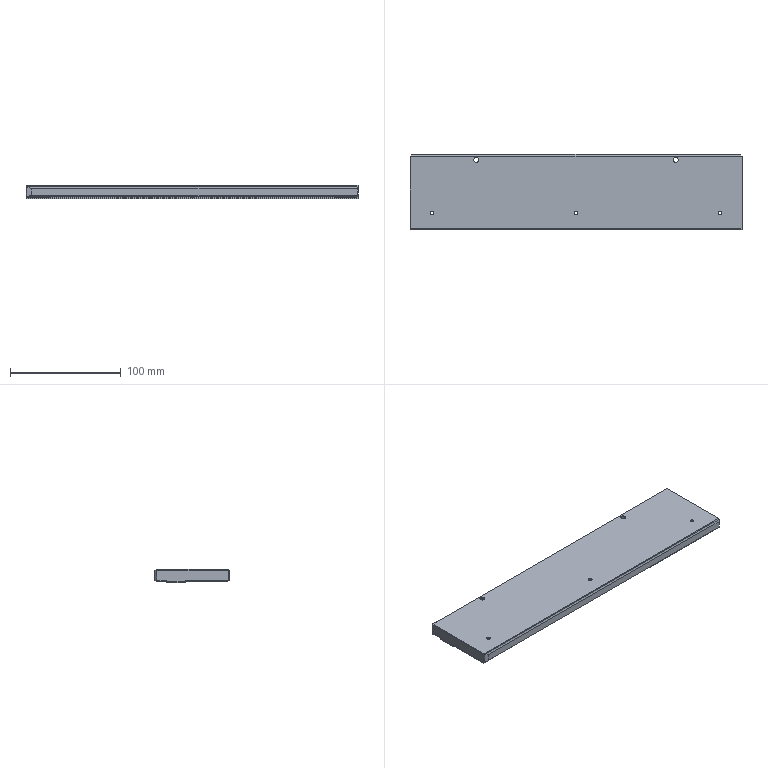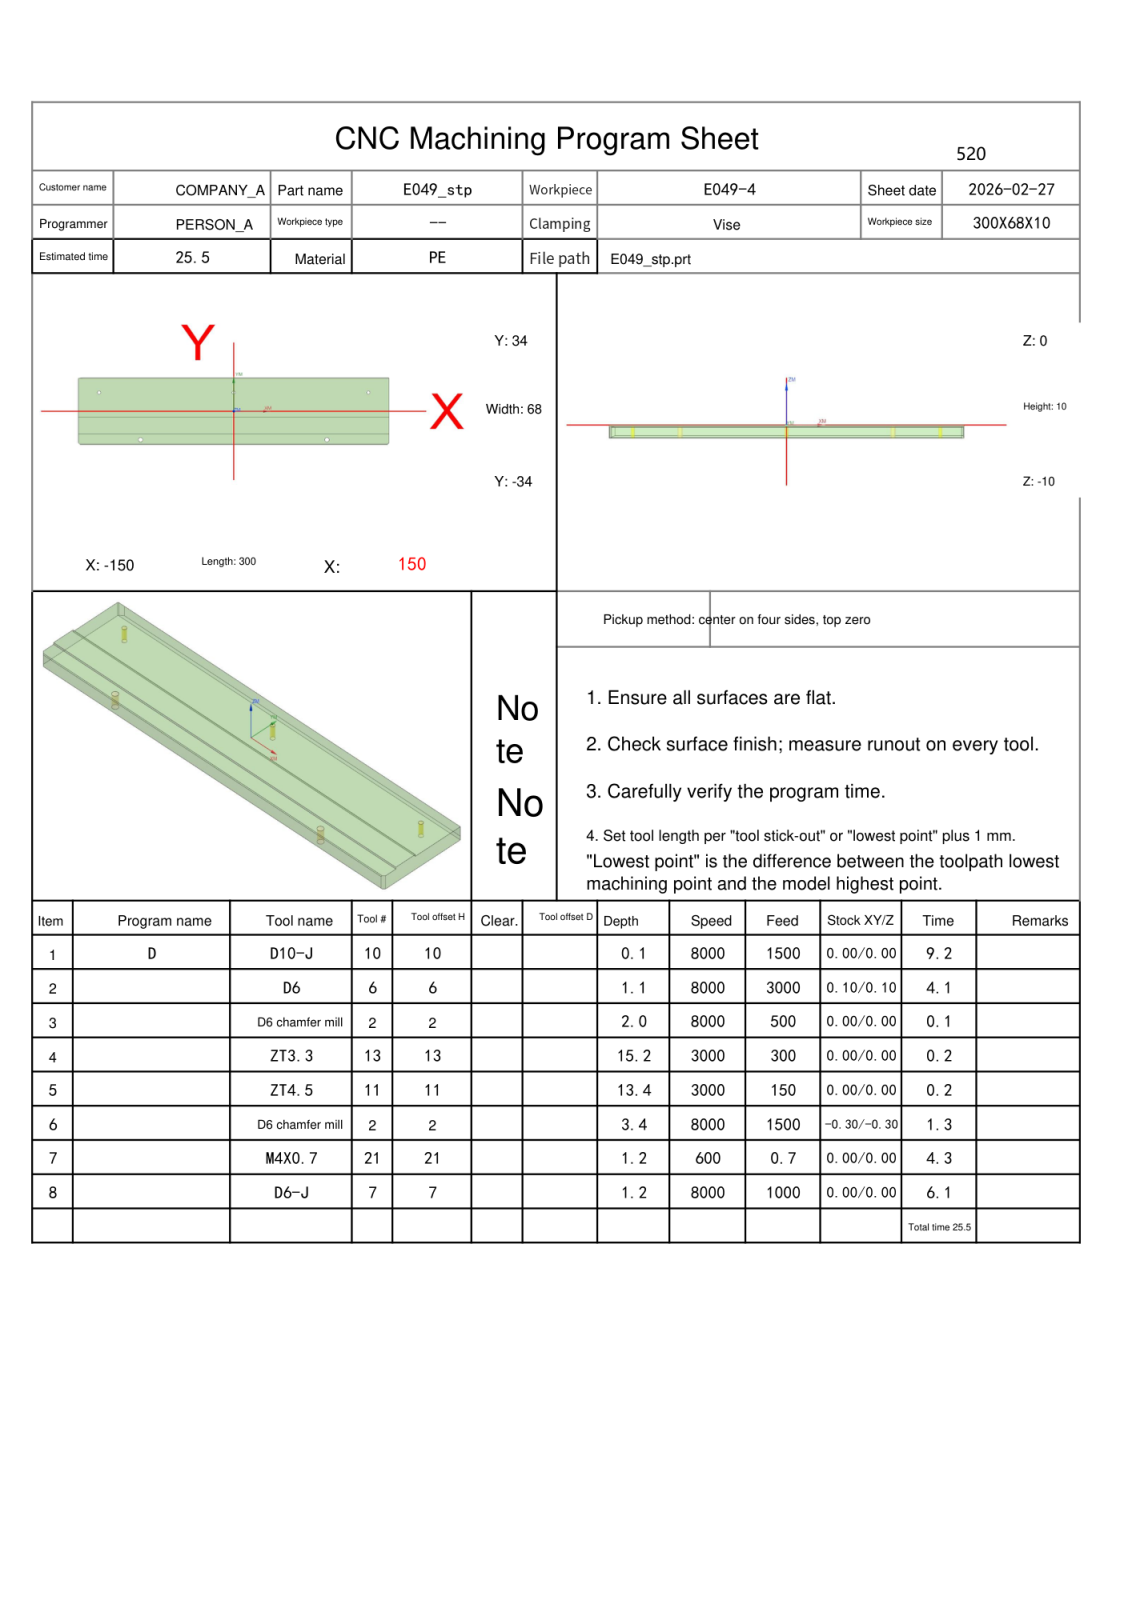NC program | NX | posted by the shop | part box 300 x 68 x 12 mm
Whole program:
%
O0001
(Machine time: 27.03 MIN)
(===Total Tool:7===)
(T10=D10-J  D=10.  R=0.   D-  H10 Z=0.    )
(T6=D6      D=6.   R=0.   D-  H06 Z=-1.1  )
(T2=D6 chamfer mill   D=6.   R=0.   D-  H02 Z=-3.37 )
(T13=ZT3.3  D=3.3  DR_a=118 D-  H13 Z=-15.2 )
(T11=ZT4.5  D=4.5  DR_a=118 D-  H11 Z=-13.35)
(T21=M4X0.7 D=3.3  DR_a=180 D-  H21 Z=-1.2  )
(T7=D6-J    D=6.   R=0.   D7  H07 Z=-1.2  )
G80 G90 G17 G49 G40
G91 G28 Z0
M01
N1 T10 M06
(D10-J  D=10. R=0. H=10 ce=0.00 di=0.10)
G00 G90 G54 X140.3 Y44. M03 S4500
G43 H10 Z30.
M08
Z2.55
G01 Z.55 F1500.
X145.3 Y39.
X155. Y29.3
Y19.6
X135.6 Y39.
X125.9
X155. Y9.9
Y.2
X116.2 Y39.
X106.5
X155. Y-9.5
Y-19.2
X96.8 Y39.
X87.1
X155. Y-28.9
Y-38.6
X77.4 Y39.
X67.7
X145.7 Y-39.
X136.
X58. Y39.
X48.3
X126.3 Y-39.
X116.6
X38.6 Y39.
X28.9
X106.9 Y-39.
X97.2
X19.2 Y39.
X9.5
X87.5 Y-39.
X77.8
X-.2 Y39.
X-9.9
X68.1 Y-39.
X58.4
X-19.6 Y39.
X-29.3
X48.7 Y-39.
X39.
X-39. Y39.
X-48.7
X29.3 Y-39.
X19.6
X-58.4 Y39.
X-68.1
X9.9 Y-39.
X.2
X-77.8 Y39.
X-87.5
X-9.5 Y-39.
X-19.2
X-97.2 Y39.
X-106.9
X-28.9 Y-39.
X-38.6
X-116.6 Y39.
X-126.3
X-48.3 Y-39.
X-58.
X-136. Y39.
X-145.7
X-67.7 Y-39.
X-77.4
X-155. Y38.6
Y28.9
X-87.1 Y-39.
X-96.8
X-155. Y19.2
Y9.5
X-106.5 Y-39.
X-116.2
X-155. Y-.2
Y-9.9
X-125.9 Y-39.
X-135.6
X-155. Y-19.6
Y-29.3
X-145.3 Y-39.
X-140.3 Y-44.
Z2.55
G00 Z4.
X160. Y24.3
Z2.1
G01 Z.1
X155. Y29.3
X145.3 Y39.
X135.6
X155. Y19.6
Y9.9
X125.9 Y39.
X116.2
X155. Y.2
Y-9.5
X106.5 Y39.
X96.8
X155. Y-19.2
Y-28.9
X87.1 Y39.
X77.4
X155. Y-38.6
Y-39.
X145.7
X67.7 Y39.
X58.
X136. Y-39.
X126.3
X48.3 Y39.
X38.6
X116.6 Y-39.
X106.9
X28.9 Y39.
X19.2
X97.2 Y-39.
X87.5
X9.5 Y39.
X-.2
X77.8 Y-39.
X68.1
X-9.9 Y39.
X-19.6
X58.4 Y-39.
X48.7
X-29.3 Y39.
X-39.
X39. Y-39.
X29.3
X-48.7 Y39.
X-58.4
X19.6 Y-39.
X9.9
X-68.1 Y39.
X-77.8
X.2 Y-39.
X-9.5
X-87.5 Y39.
X-97.2
X-19.2 Y-39.
X-28.9
X-106.9 Y39.
X-116.6
X-38.6 Y-39.
X-48.3
X-126.3 Y39.
X-136.
X-58. Y-39.
X-67.7
X-145.7 Y39.
X-155.
Y38.6
X-77.4 Y-39.
X-87.1
X-155. Y28.9
Y19.2
X-96.8 Y-39.
X-106.5
X-155. Y9.5
Y-.2
X-116.2 Y-39.
X-125.9
X-155. Y-9.9
Y-19.6
X-135.6 Y-39.
X-145.3
X-155. Y-29.3
X-160. Y-24.3
Z2.1
G00 Z30.
G00 G90 X-167. Y17.3 M03 S8000
Z30.
Z2.
G01 Z0.0 F1000.
X-155. Y29.3
X-145.3 Y39.
X-135.6
X-155. Y19.6
Y9.9
X-125.9 Y39.
X-116.2
X-155. Y.2
Y-9.5
X-106.5 Y39.
X-96.8
X-155. Y-19.2
Y-28.9
X-87.1 Y39.
X-77.4
X-155. Y-38.6
Y-39.
X-145.7
X-67.7 Y39.
X-58.
X-136. Y-39.
X-126.3
X-48.3 Y39.
X-38.6
X-116.6 Y-39.
X-106.9
X-28.9 Y39.
X-19.2
X-97.2 Y-39.
X-87.5
X-9.5 Y39.
X.2
X-77.8 Y-39.
X-68.1
X9.9 Y39.
X19.6
X-58.4 Y-39.
X-48.7
X29.3 Y39.
X39.
X-39. Y-39.
X-29.3
X48.7 Y39.
X58.4
X-19.6 Y-39.
X-9.9
X68.1 Y39.
X77.8
X-.2 Y-39.
X9.5
X87.5 Y39.
X97.2
X19.2 Y-39.
X28.9
X106.9 Y39.
X116.6
X38.6 Y-39.
X48.3
X126.3 Y39.
X136.
X58. Y-39.
X67.7
X145.7 Y39.
X155.
Y38.6
X77.4 Y-39.
X87.1
X155. Y28.9
Y19.2
X96.8 Y-39.
X106.5
X155. Y9.5
Y-.2
X116.2 Y-39.
X125.9
X155. Y-9.9
Y-19.6
X135.6 Y-39.
X145.3
X155. Y-29.3
X167. Y-17.3
Z2.
G00 Z30.
G91 G28 Z0.0
M05
M09
G91 G28 Z0.0
M01
N2 T06 M06
(D6  D=6. R=0. H=06 ce=0.10 di=0.10)
G00 G90 G54 X156. Y36.1 M03 S8000
G43 H06 Z11.
M08
Z1.133
G01 Z-.367 F3000.
X152.94
X-150.894
G03 X-151.338 Y35.903 I.001 J-.6
G01 X-152.785 Y34.304
G03 X-152.94 Y33.902 I.445 J-.402
G01 Y33.699
G03 X-152.341 Y33.1 I.6 J.001
G01 X152.341
G02 X152.94 Y32.501 I-.001 J-.6
G01 Y29.199
G02 X152.341 Y28.6 I-.6 J.001
G01 X-152.341
G03 X-152.94 Y28.001 I.001 J-.6
G01 Y24.699
G03 X-152.341 Y24.1 I.6 J.001
G01 X152.341
G02 X152.94 Y23.501 I-.001 J-.6
G01 Y20.199
G02 X152.341 Y19.6 I-.6 J.001
G01 X-152.341
G03 X-152.94 Y19.001 I.001 J-.6
G01 Y15.699
G03 X-152.341 Y15.1 I.6 J.001
G01 X152.341
G02 X152.94 Y14.501 I-.001 J-.6
G01 Y11.199
G02 X152.341 Y10.6 I-.6 J.001
G01 X-152.341
G03 X-152.94 Y10.001 I.001 J-.6
G01 Y6.699
G03 X-152.341 Y6.1 I.6 J.001
G01 X152.341
G02 X152.94 Y5.501 I-.001 J-.6
G01 Y2.199
G02 X152.341 Y1.6 I-.6 J.001
G01 X-152.427
G03 X-153.019 Y1.093 I.001 J-.6
G01 X-153.533 Y-2.208
X-153.54 Y-2.3
G03 X-152.94 Y-2.9 I.6 J0.0
G01 X152.94
X156.1
Z1.133
G00 X156. Y36.1
Z.767
G01 Z-.733
X152.94
X-150.894
G03 X-151.338 Y35.903 I.001 J-.6
G01 X-152.785 Y34.304
G03 X-152.94 Y33.902 I.445 J-.402
G01 Y33.699
G03 X-152.341 Y33.1 I.6 J.001
G01 X152.341
G02 X152.94 Y32.501 I-.001 J-.6
G01 Y29.199
G02 X152.341 Y28.6 I-.6 J.001
G01 X-152.341
G03 X-152.94 Y28.001 I.001 J-.6
G01 Y24.699
G03 X-152.341 Y24.1 I.6 J.001
G01 X152.341
G02 X152.94 Y23.501 I-.001 J-.6
G01 Y20.199
G02 X152.341 Y19.6 I-.6 J.001
G01 X-152.341
G03 X-152.94 Y19.001 I.001 J-.6
G01 Y15.699
G03 X-152.341 Y15.1 I.6 J.001
G01 X152.341
G02 X152.94 Y14.501 I-.001 J-.6
G01 Y11.199
G02 X152.341 Y10.6 I-.6 J.001
G01 X-152.341
G03 X-152.94 Y10.001 I.001 J-.6
G01 Y6.699
G03 X-152.341 Y6.1 I.6 J.001
G01 X152.341
G02 X152.94 Y5.501 I-.001 J-.6
G01 Y2.199
G02 X152.341 Y1.6 I-.6 J.001
G01 X-152.427
G03 X-153.019 Y1.093 I.001 J-.6
G01 X-153.533 Y-2.208
X-153.54 Y-2.3
G03 X-152.94 Y-2.9 I.6 J0.0
G01 X152.94
X156.1
Z.767
G00 X156. Y36.1
Z.4
G01 Z-1.1
X152.94
X-150.894
G03 X-151.338 Y35.903 I.001 J-.6
G01 X-152.785 Y34.304
G03 X-152.94 Y33.902 I.445 J-.402
G01 Y33.699
G03 X-152.341 Y33.1 I.6 J.001
G01 X152.341
G02 X152.94 Y32.501 I-.001 J-.6
G01 Y29.199
G02 X152.341 Y28.6 I-.6 J.001
G01 X-152.341
G03 X-152.94 Y28.001 I.001 J-.6
G01 Y24.699
G03 X-152.341 Y24.1 I.6 J.001
G01 X152.341
G02 X152.94 Y23.501 I-.001 J-.6
G01 Y20.199
G02 X152.341 Y19.6 I-.6 J.001
G01 X-152.341
G03 X-152.94 Y19.001 I.001 J-.6
G01 Y15.699
G03 X-152.341 Y15.1 I.6 J.001
G01 X152.341
G02 X152.94 Y14.501 I-.001 J-.6
G01 Y11.199
G02 X152.341 Y10.6 I-.6 J.001
G01 X-152.341
G03 X-152.94 Y10.001 I.001 J-.6
G01 Y6.699
G03 X-152.341 Y6.1 I.6 J.001
G01 X152.341
G02 X152.94 Y5.501 I-.001 J-.6
G01 Y2.199
G02 X152.341 Y1.6 I-.6 J.001
G01 X-152.427
G03 X-153.019 Y1.093 I.001 J-.6
G01 X-153.533 Y-2.208
X-153.54 Y-2.3
G03 X-152.94 Y-2.9 I.6 J0.0
G01 X152.94
X156.1
Z.4
G00 Z3.
X155.353 Y-35.1
Z1.133
G01 Z-.367
X151.058
X-150.81
G02 X-151.233 Y-34.925 I.001 J.6
G01 X-152.764 Y-33.393
G02 X-152.94 Y-32.969 I.424 J.424
G01 Y-31.199
G02 X-152.341 Y-30.6 I.6 J-.001
G01 X152.427
G03 X153.019 Y-30.093 I-.001 J.6
G01 X153.533 Y-26.792
X153.54 Y-26.7
G03 X152.94 Y-26.1 I-.6 J0.0
G01 X-152.94
X-156.1
Z1.133
G00 X155.353 Y-35.1
Z.767
G01 Z-.733
X151.058
X-150.81
G02 X-151.233 Y-34.925 I.001 J.6
G01 X-152.764 Y-33.393
G02 X-152.94 Y-32.969 I.424 J.424
G01 Y-31.199
G02 X-152.341 Y-30.6 I.6 J-.001
G01 X152.427
G03 X153.019 Y-30.093 I-.001 J.6
G01 X153.533 Y-26.792
X153.54 Y-26.7
G03 X152.94 Y-26.1 I-.6 J0.0
G01 X-152.94
X-156.1
Z.767
G00 X155.353 Y-35.1
Z.4
G01 Z-1.1
X151.058
X-150.81
G02 X-151.233 Y-34.925 I.001 J.6
G01 X-152.764 Y-33.393
G02 X-152.94 Y-32.969 I.424 J.424
G01 Y-31.199
G02 X-152.341 Y-30.6 I.6 J-.001
G01 X152.427
G03 X153.019 Y-30.093 I-.001 J.6
G01 X153.533 Y-26.792
X153.54 Y-26.7
G03 X152.94 Y-26.1 I-.6 J0.0
G01 X-152.94
X-156.1
Z.4
G00 Z11.
G91 G28 Z0.0
M05
M09
G91 G28 Z0.0
M01
N3 T02 M06
(D6 chamfer mill  D=6. R=0. H=02 ce=0.00 di=0.10)
G00 G90 G54 X130. Y19. M03 S8000
G43 H02 Z30.
M08
G98 G81 X130. Y19. Z-2. R-.2 F500.
X90. Y-29.
X0.0 Y19.
X-90. Y-29.
X-130. Y19.
G80
G00 Z30.
G91 G28 Z0.0
M05
M09
G91 G28 Z0.0
M01
N4 T13 M06
(ZT3.3 D=3.3 DR_a=118 H=13)
G00 G90 G54 X130. Y19. M03 S3000
G43 H13 Z30.
M08
G98 G83 X130. Y19. Z-15.2 R-.2 F300. Q2.
X0.0
X-130.
G80
G00 Z30.
G91 G28 Z0.0
M05
M09
G91 G28 Z0.0
M01
N5 T11 M06
(ZT4.5 D=4.5 DR_a=118 H=11)
G00 G90 G54 X-90. Y-29. M03 S3000
G43 H11 Z30.
M08
G98 G83 X-90. Y-29. Z-13.352 R-.2 F150. Q3.
X90.
G80
G00 Z30.
G91 G28 Z0.0
M05
M09
G91 G28 Z0.0
M01
N6 T02 M06
(D6 chamfer mill  D=6. R=0. H=02 ce=0.00 di=0.10)
G00 G90 G54 X130. Y19. M03 S8000
G43 H02 Z30.
M08
G98 G81 X130. Y19. Z-3.371 R1.8 F500.
X0.0
X-130.
G80
G00 Z30.
G00 G90 X-89.982 Y-29.55 M03 S8000
Z30.
Z-1.7
G01 Z-2.2 F500.
X-89.95 Y-30.5
G03 X-88.45 Y-29. I0.0 J1.5
X-90. Y-27.45 I-1.55 J0.0
X-91.55 Y-29. I0.0 J-1.55
X-90. Y-30.55 I1.55 J0.0
X-88.45 Y-29. I0.0 J1.55
X-89.95 Y-27.5 I-1.5 J0.0
G01 X-89.982 Y-28.45
Z-1.7
G00 Z30.
X90.018 Y-29.55
Z-1.7
G01 Z-2.2
X90.05 Y-30.5
G03 X91.55 Y-29. I0.0 J1.5
X90. Y-27.45 I-1.55 J0.0
X88.45 Y-29. I0.0 J-1.55
X90. Y-30.55 I1.55 J0.0
X91.55 Y-29. I0.0 J1.55
X90.05 Y-27.5 I-1.5 J0.0
G01 X90.018 Y-28.45
Z-1.7
G00 Z30.
G00 G90 X.386 Y-23.827 M03 S6500
Z30.
Z.572
G01 Z-.8 F1500.
G03 X.1 Y-23.627 I-1.286 J-1.532
G01 X.054 Y-23.597
X0.0 Y-23.6
X-150.
G02 X-150.6 Y-23. I0.0 J.6
G01 Y-6.
G02 X-150. Y-5.4 I.6 J0.0
G01 X150.
G02 X150.6 Y-6. I0.0 J-.6
G01 Y-23.
G02 X150. Y-23.6 I-.6 J0.0
G01 X0.0
X-.054 Y-23.597
X-.1 Y-23.627
G03 X-.386 Y-23.827 I1. J-1.732
G01 Z.572
G00 Z10.
X150.6 Y-24.898
Z2.
G01 Z-2.
Y-32.
X150.58 Y-32.155
X150.52 Y-32.3
X150.424 Y-32.424
X148.924 Y-33.924
X148.8 Y-34.02
X148.691 Y-34.065
X148.667 Y-34.083
X148.611 Y-34.172
Z-.482
G00 Z10.
X-148.611
Z-.482
G01 Z-2.
X-148.667 Y-34.083
X-148.691 Y-34.065
X-148.8 Y-34.02
X-148.924 Y-33.924
X-150.424 Y-32.424
X-150.52 Y-32.3
X-150.58 Y-32.155
X-150.6 Y-32.
Y-24.898
Z2.
G00 Z10.
X-88.535 Y-29.407
Z-.521
G01 Z-2.
G03 X-88.366 Y-29.102 I-1.658 J1.118
G01 X-88.341 Y-29.054
X-88.35 Y-29.
G03 X-90. Y-27.35 I-1.65 J0.0
X-91.65 Y-29. I0.0 J-1.65
X-90. Y-30.65 I1.65 J0.0
X-88.35 Y-29. I0.0 J1.65
G01 X-88.341 Y-28.946
X-88.366 Y-28.898
G03 X-88.535 Y-28.593 I-1.827 J-.813
G01 Z-.521
G00 Z10.
X91.465 Y-29.407
Z-.521
G01 Z-2.
G03 X91.634 Y-29.102 I-1.658 J1.118
G01 X91.659 Y-29.054
X91.65 Y-29.
G03 X90. Y-27.35 I-1.65 J0.0
X88.35 Y-29. I0.0 J-1.65
X90. Y-30.65 I1.65 J0.0
X91.65 Y-29. I0.0 J1.65
G01 X91.659 Y-28.946
X91.634 Y-28.898
G03 X91.465 Y-28.593 I-1.827 J-.813
G01 Z-.521
G00 Z10.
X-150.6 Y-4.096
Z2.
G01 Z-2.
Y33.
X-150.582 Y33.146
X-150.529 Y33.283
X-150.445 Y33.403
X-149.992 Y33.903
X-149.865 Y34.009
X-149.712 Y34.077
X-149.548 Y34.1
X-149.292
Z2.
G00 Z10.
X149.993 Y34.372
Z-.674
G01 Z-2.
G03 X150.124 Y34.126 I1.473 J.625
G01 X150.144 Y34.087
X150.185 Y34.071
X150.353 Y33.985
X150.485 Y33.853
X150.571 Y33.685
X150.6 Y33.5
Y-4.11
Z2.
G00 Z10.
X-129.153 Y18.588
Z-.475
G01 Z-2.
G03 X-128.993 Y18.897 I-1.687 J1.075
G01 X-128.969 Y18.946
X-128.979 Y19.
G03 X-130. Y20.021 I-1.021 J0.0
X-131.021 Y19. I0.0 J-1.021
X-130. Y17.979 I1.021 J0.0
X-128.979 Y19. I0.0 J1.021
G01 X-128.969 Y19.054
X-128.993 Y19.103
G03 X-129.153 Y19.412 I-1.848 J-.765
G01 Z-.475
G00 Z10.
X.847 Y18.588
Z-.475
G01 Z-2.
G03 X1.007 Y18.897 I-1.687 J1.075
G01 X1.031 Y18.946
X1.021 Y19.
G03 X0.0 Y20.021 I-1.021 J0.0
X-1.021 Y19. I0.0 J-1.021
X0.0 Y17.979 I1.021 J0.0
X1.021 Y19. I0.0 J1.021
G01 X1.031 Y19.054
X1.007 Y19.103
G03 X.847 Y19.412 I-1.848 J-.765
G01 Z-.475
G00 Z10.
X130.847 Y18.588
Z-.475
G01 Z-2.
G03 X131.007 Y18.897 I-1.687 J1.075
G01 X131.031 Y18.946
X131.021 Y19.
G03 X130. Y20.021 I-1.021 J0.0
X128.979 Y19. I0.0 J-1.021
X130. Y17.979 I1.021 J0.0
X131.021 Y19. I0.0 J1.021
G01 X131.031 Y19.054
X131.007 Y19.103
G03 X130.847 Y19.412 I-1.848 J-.765
G01 Z-.475
G00 Z30.
G00 G90 X152.407 Y-35.9 M03 S6500
Z30.
Z-.9
G01 Z-2.4 F1500.
G03 X151.207 Y-34.7 I-1.2 J0.0
G01 X-151.207
G03 X-152.407 Y-35.9 I0.0 J-1.2
G01 Z-.9
G00 Z30.
X-153.388 Y35.9
Z-.9
G01 Z-2.4
G03 X-152.188 Y34.7 I1.2 J0.0
G01 X152.707
G03 X153.907 Y35.9 I0.0 J1.2
G01 Z-.9
G00 Z30.
G91 G28 Z0.0
M05
M09
G91 G28 Z0.0
M01
N7 T21 M06
(M4X0.7 D=3.3 DR_a=180 H=21)
G00 G90 G54 X130. Y19. M03 S600
G43 H21 Z30.
M08
G95
G98 G84 X130. Y19. Z-1.2 R-.2 F.7 Q4.
X0.0
X-130.
G80
G94
G00 Z30.
G91 G28 Z0.0
M05
M09
G91 G28 Z0.0
M01
N8 T07 M06
(D6-J  D=6. R=0. H=07 ce=0.40 di=0.00)
G00 G90 G54 X-1.2 Y37.7 M03 S8000
G43 H07 Z11.
M08
Z.3
G01 Z-1.2 F1000.
Y35.3
G03 X0.0 Y34.1 I1.2 J0.0
G01 X150.004
G02 X150.6 Y33.504 I-.004 J-.6
G01 Y-2.004
G02 X150.004 Y-2.6 I-.6 J.004
G01 X-150.004
G02 X-150.6 Y-2.004 I.004 J.6
G01 Y33.004
G02 X-150.447 Y33.4 I.6 J-.004
G01 X-149.99 Y33.905
G02 X-149.551 Y34.1 I.442 J-.405
G01 X1.252
G02 X1.675 Y33.925 I-.001 J-.6
G01 X4.325 Y31.275
G03 X4.748 Y31.1 I.424 J.425
G01 X147.004
G02 X147.6 Y30.504 I-.004 J-.6
G01 Y.996
G02 X147.004 Y.4 I-.6 J.004
G01 X-147.004
G02 X-147.6 Y.996 I.004 J.6
G01 Y30.504
G02 X-147.004 Y31.1 I.6 J-.004
G01 X1.252
G02 X1.675 Y30.925 I-.001 J-.6
G01 X4.325 Y28.275
G03 X4.748 Y28.1 I.424 J.425
G01 X144.004
G02 X144.6 Y27.504 I-.004 J-.6
G01 Y3.996
G02 X144.004 Y3.4 I-.6 J.004
G01 X-144.004
G02 X-144.6 Y3.996 I.004 J.6
G01 Y27.504
G02 X-144.004 Y28.1 I.6 J-.004
G01 X1.252
G02 X1.675 Y27.925 I-.001 J-.6
G01 X4.325 Y25.275
G03 X4.748 Y25.1 I.424 J.425
G01 X141.005
G02 X141.6 Y24.505 I-.005 J-.6
G01 Y6.995
G02 X141.005 Y6.4 I-.6 J.005
G01 X-141.005
G02 X-141.6 Y6.995 I.005 J.6
G01 Y24.505
G02 X-141.005 Y25.1 I.6 J-.005
G01 X1.252
G02 X1.675 Y24.925 I-.001 J-.6
G01 X4.325 Y22.275
G03 X4.748 Y22.1 I.424 J.425
G01 X138.005
G02 X138.6 Y21.505 I-.005 J-.6
G01 Y9.995
G02 X138.005 Y9.4 I-.6 J.005
G01 X-138.005
G02 X-138.6 Y9.995 I.005 J.6
G01 Y21.505
G02 X-138.005 Y22.1 I.6 J-.005
G01 X1.252
G02 X1.675 Y21.925 I-.001 J-.6
G01 X4.325 Y19.275
G03 X4.748 Y19.1 I.424 J.425
G01 X135.005
G02 X135.6 Y18.505 I-.005 J-.6
G01 Y12.995
G02 X135.005 Y12.4 I-.6 J.005
G01 X-135.005
G02 X-135.6 Y12.995 I.005 J.6
G01 Y18.505
G02 X-135.005 Y19.1 I.6 J-.005
G01 X1.252
G02 X1.675 Y18.925 I-.001 J-.6
G01 X4.325 Y16.275
G03 X4.748 Y16.1 I.424 J.425
G01 X132.304
G02 X132.6 Y15.804 I-.004 J-.3
G01 Y15.696
G02 X132.304 Y15.4 I-.3 J.004
G01 X-132.304
G02 X-132.6 Y15.696 I.004 J.3
G01 Y15.804
G02 X-132.304 Y16.1 I.3 J-.004
G01 X3.
X4.
G03 X5.2 Y17.3 I0.0 J1.2
G01 Z.3
G00 Z11.
X1.2 Y-37.7
Z.3
G01 Z-1.2
Y-35.3
G03 X0.0 Y-34.1 I-1.2 J0.0
G01 X-148.504
G02 X-148.922 Y-33.927 I.004 J.6
G01 X-150.427 Y-32.422
G02 X-150.6 Y-32.004 I.427 J.422
G01 Y-26.996
G02 X-150.004 Y-26.4 I.6 J-.004
G01 X150.004
G02 X150.6 Y-26.996 I-.004 J-.6
G01 Y-32.004
G02 X150.427 Y-32.422 I-.6 J.004
G01 X148.922 Y-33.927
G02 X148.504 Y-34.1 I-.422 J.427
G01 X-3.
G02 X-3.565 Y-33.703 I0.0 J.6
G01 X-4.358 Y-31.496
G03 X-4.921 Y-31.1 I-.564 J-.204
G01 X-147.004
G02 X-147.6 Y-30.504 I.004 J.6
G01 Y-29.996
G02 X-147.004 Y-29.4 I.6 J-.004
G01 X147.004
G02 X147.6 Y-29.996 I-.004 J-.6
G01 Y-30.504
G02 X147.004 Y-31.1 I-.6 J.004
G01 X-3.
X-4.
G03 X-5.2 Y-32.3 I0.0 J-1.2
G01 Y-37.7
Z.3
G00 Z11.
G00 G90 X-154.2 Y-1.601 M03 S8000
Z11.
Z-.2
G01 Z-1.2 F1000.
G41 D07
Y-1.801
G03 X-153. Y-3. I1.2 J.001
G01 X153.
G03 X154.2 Y-1.801 I0.0 J1.2
G01 G40 Y-1.601
Z-.2
G00 Z3.8
Y-27.399
Z-.2
G01 Z-1.2
G41 D07
Y-27.199
G03 X153. Y-26. I-1.2 J-.001
G01 X-153.
G03 X-154.2 Y-27.199 I0.0 J-1.2
G01 G40 Y-27.399
Z-.2
G00 Z11.
M05
M09
G91 G28 Z0.0
G91 G28 Y0.0
M30
%